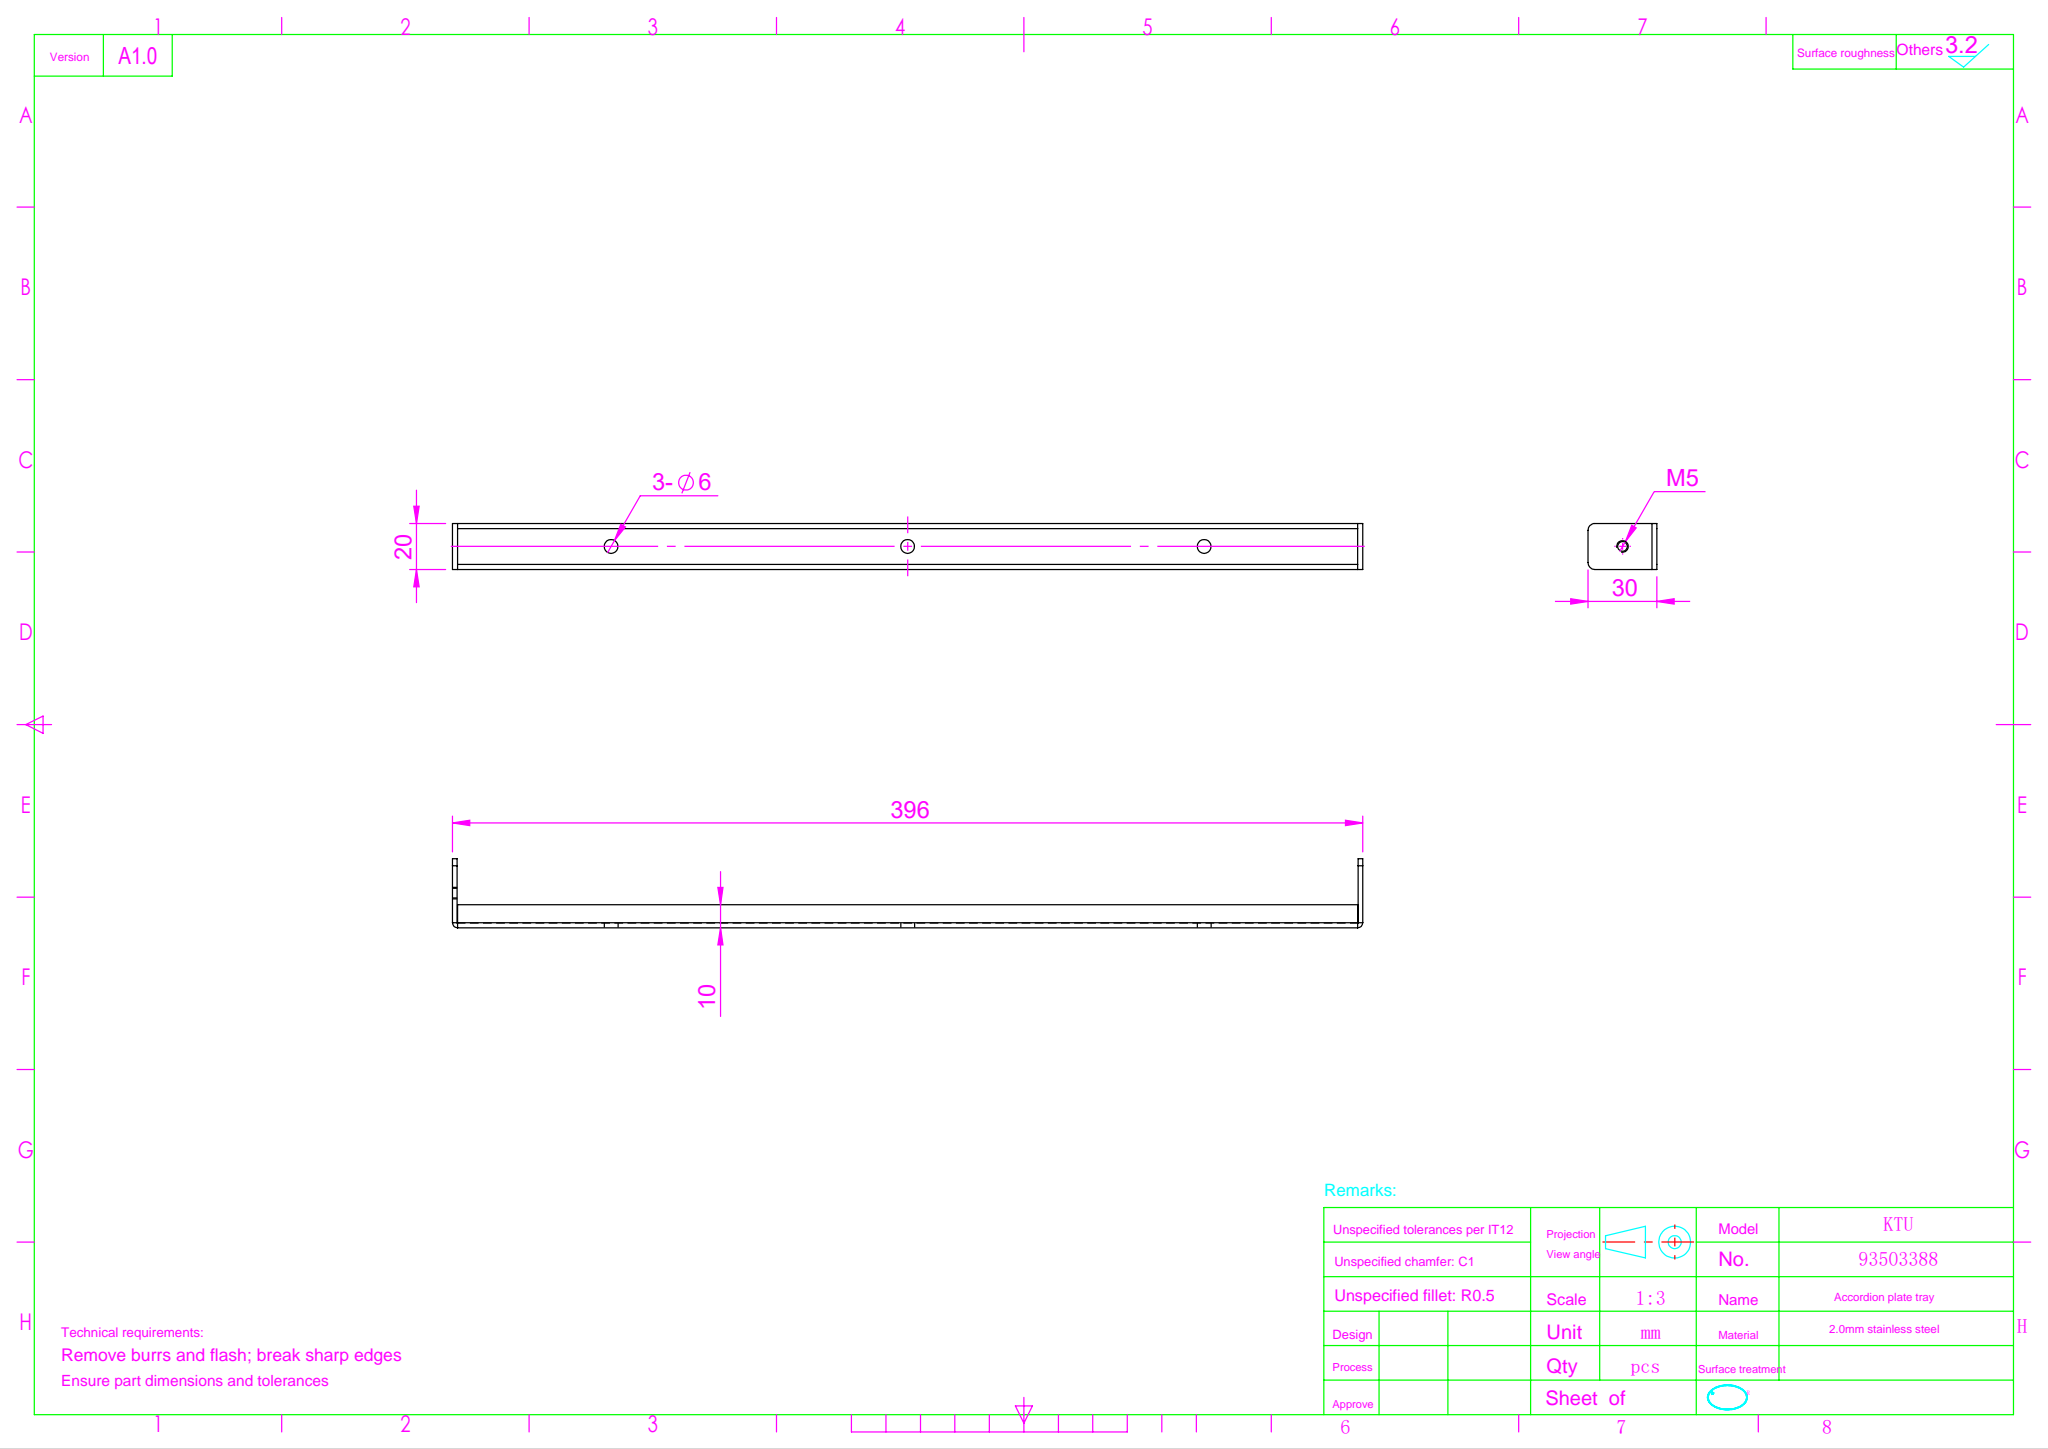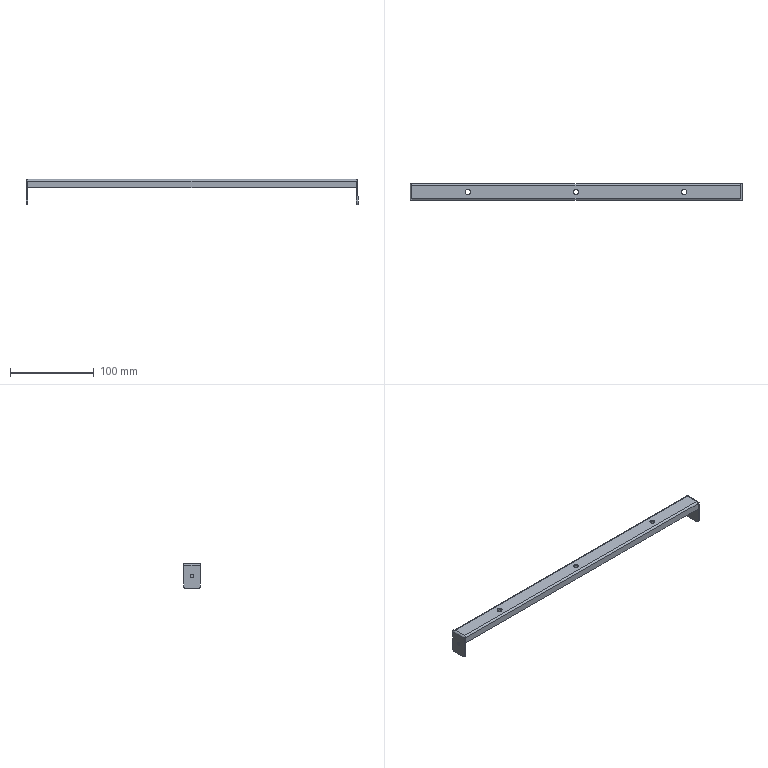Part | SolidWorks | features EdgeFlange 2, Fillet 1, FlatPattern 1, ICE 1, SMBaseFlange 1, SheetMetal 1 | 1 solid | 54 faces | box 396 x 20 x 30 mm | volume 29550 mm3 | plane 34 | cylinder 20 | commonest cylinder face diameters 6 x10 0.4 x4 4.4 x4 4.2 x2